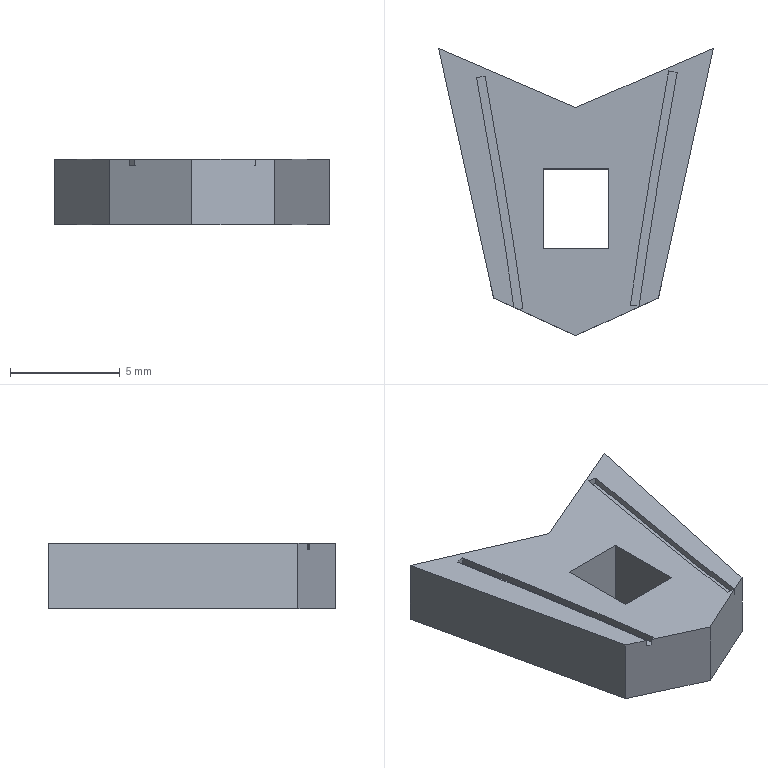Part | SolidWorks | features BaseBody 1 | 1 solid | 22 faces | box 12.536 x 13.11 x 3 mm | volume 276.053 mm3 | plane 18 | spline 4
STEP:
#1=CARTESIAN_POINT('',(2.822,-5.905,1.2));
#2=VERTEX_POINT('',#1);
#3=CARTESIAN_POINT('',(1.08,-16.586,1.2));
#4=VERTEX_POINT('',#3);
#5=CARTESIAN_POINT('',(2.822,-5.905,1.2));
#6=CARTESIAN_POINT('',(2.422,-8.09,1.2));
#7=CARTESIAN_POINT('',(1.593,-12.754,1.2));
#8=CARTESIAN_POINT('',(1.08,-16.586,1.2));
#9=B_SPLINE_CURVE_WITH_KNOTS('',3,(#5,#6,#7,#8),.UNSPECIFIED.,.F.,.F.,(4,4),(0.2382,0.9072),.UNSPECIFIED.);
#10=EDGE_CURVE('',#2,#4,#9,.T.);
#11=ORIENTED_EDGE('',*,*,#10,.T.);
#12=CARTESIAN_POINT('',(1.476,-16.639,1.2));
#13=VERTEX_POINT('',#12);
#14=CARTESIAN_POINT('',(1.476,-16.639,1.2));
#15=DIRECTION('',(-0.9911,0.1328,0.));
#16=VECTOR('',#15,1000.);
#17=LINE('',#14,#16);
#18=EDGE_CURVE('',#13,#4,#17,.T.);
#19=ORIENTED_EDGE('',*,*,#18,.F.);
#20=CARTESIAN_POINT('',(3.216,-5.977,1.2));
#21=VERTEX_POINT('',#20);
#22=CARTESIAN_POINT('',(3.216,-5.977,1.2));
#23=CARTESIAN_POINT('',(2.816,-8.159,1.2));
#24=CARTESIAN_POINT('',(1.988,-12.821,1.2));
#25=CARTESIAN_POINT('',(1.476,-16.639,1.2));
#26=B_SPLINE_CURVE_WITH_KNOTS('',3,(#22,#23,#24,#25),.UNSPECIFIED.,.F.,.F.,(4,4),(0.,1.),.UNSPECIFIED.);
#27=EDGE_CURVE('',#21,#13,#26,.T.);
#28=ORIENTED_EDGE('',*,*,#27,.F.);
#29=CARTESIAN_POINT('',(2.822,-5.905,1.2));
#30=DIRECTION('',(0.9837,-0.18,0.));
#31=VECTOR('',#30,1000.);
#32=LINE('',#29,#31);
#33=EDGE_CURVE('',#2,#21,#32,.T.);
#34=ORIENTED_EDGE('',*,*,#33,.F.);
#35=EDGE_LOOP('',(#11,#19,#28,#34));
#36=FACE_OUTER_BOUND('',#35,.T.);
#37=CARTESIAN_POINT('',(1.994,-10.628,1.2));
#38=DIRECTION('',(0.,0.,-1.));
#39=DIRECTION('',(0.,-1.,0.));
#40=AXIS2_PLACEMENT_3D('',#37,#38,#39);
#41=PLANE('',#40);
#42=ADVANCED_FACE('',(#36),#41,.F.);
#43=CARTESIAN_POINT('',(1.476,-16.639,1.5));
#44=VERTEX_POINT('',#43);
#45=CARTESIAN_POINT('',(1.08,-16.586,1.5));
#46=VERTEX_POINT('',#45);
#47=CARTESIAN_POINT('',(1.476,-16.639,1.5));
#48=DIRECTION('',(-0.9911,0.1328,0.));
#49=VECTOR('',#48,1000.);
#50=LINE('',#47,#49);
#51=EDGE_CURVE('',#44,#46,#50,.T.);
#52=ORIENTED_EDGE('',*,*,#51,.F.);
#53=CARTESIAN_POINT('',(1.476,-16.639,1.2));
#54=DIRECTION('',(0.,0.,1.));
#55=VECTOR('',#54,1000.);
#56=LINE('',#53,#55);
#57=EDGE_CURVE('',#13,#44,#56,.T.);
#58=ORIENTED_EDGE('',*,*,#57,.F.);
#59=ORIENTED_EDGE('',*,*,#18,.T.);
#60=CARTESIAN_POINT('',(1.08,-16.586,1.2));
#61=DIRECTION('',(0.,0.,1.));
#62=VECTOR('',#61,1000.);
#63=LINE('',#60,#62);
#64=EDGE_CURVE('',#4,#46,#63,.T.);
#65=ORIENTED_EDGE('',*,*,#64,.T.);
#66=EDGE_LOOP('',(#52,#58,#59,#65));
#67=FACE_OUTER_BOUND('',#66,.T.);
#68=CARTESIAN_POINT('',(1.476,-16.639,1.2));
#69=DIRECTION('',(0.1328,0.9911,0.));
#70=DIRECTION('',(0.,0.,-1.));
#71=AXIS2_PLACEMENT_3D('',#68,#69,#70);
#72=PLANE('',#71);
#73=ADVANCED_FACE('',(#67),#72,.T.);
#74=CARTESIAN_POINT('',(3.216,-5.977,1.5));
#75=VERTEX_POINT('',#74);
#76=CARTESIAN_POINT('',(3.216,-5.977,1.5));
#77=CARTESIAN_POINT('',(2.816,-8.159,1.5));
#78=CARTESIAN_POINT('',(1.988,-12.821,1.5));
#79=CARTESIAN_POINT('',(1.476,-16.639,1.5));
#80=B_SPLINE_CURVE_WITH_KNOTS('',3,(#76,#77,#78,#79),.UNSPECIFIED.,.F.,.F.,(4,4),(0.,1.),.UNSPECIFIED.);
#81=EDGE_CURVE('',#75,#44,#80,.T.);
#82=ORIENTED_EDGE('',*,*,#81,.F.);
#83=CARTESIAN_POINT('',(3.216,-5.977,1.2));
#84=DIRECTION('',(0.,0.,1.));
#85=VECTOR('',#84,1000.);
#86=LINE('',#83,#85);
#87=EDGE_CURVE('',#21,#75,#86,.T.);
#88=ORIENTED_EDGE('',*,*,#87,.F.);
#89=ORIENTED_EDGE('',*,*,#27,.T.);
#90=ORIENTED_EDGE('',*,*,#57,.T.);
#91=EDGE_LOOP('',(#82,#88,#89,#90));
#92=FACE_OUTER_BOUND('',#91,.T.);
#93=CARTESIAN_POINT('',(3.216,-5.977,1.2));
#94=CARTESIAN_POINT('',(3.216,-5.977,1.5));
#95=CARTESIAN_POINT('',(2.816,-8.159,1.2));
#96=CARTESIAN_POINT('',(2.816,-8.159,1.5));
#97=CARTESIAN_POINT('',(1.988,-12.821,1.2));
#98=CARTESIAN_POINT('',(1.988,-12.821,1.5));
#99=CARTESIAN_POINT('',(1.476,-16.639,1.2));
#100=CARTESIAN_POINT('',(1.476,-16.639,1.5));
#101=B_SPLINE_SURFACE_WITH_KNOTS('',3,1,((#93,#94),(#95,#96),(#97,#98),(#99,#100)),.UNSPECIFIED.,.F.,.F.,.F.,(4,4),(2,2),(0.,1.),(0.,1.),.UNSPECIFIED.);
#102=ADVANCED_FACE('',(#92),#101,.T.);
#103=CARTESIAN_POINT('',(2.822,-5.905,1.5));
#104=VERTEX_POINT('',#103);
#105=CARTESIAN_POINT('',(2.822,-5.905,1.5));
#106=DIRECTION('',(0.9837,-0.18,0.));
#107=VECTOR('',#106,1000.);
#108=LINE('',#105,#107);
#109=EDGE_CURVE('',#104,#75,#108,.T.);
#110=ORIENTED_EDGE('',*,*,#109,.F.);
#111=CARTESIAN_POINT('',(2.822,-5.905,1.2));
#112=DIRECTION('',(0.,0.,1.));
#113=VECTOR('',#112,1000.);
#114=LINE('',#111,#113);
#115=EDGE_CURVE('',#2,#104,#114,.T.);
#116=ORIENTED_EDGE('',*,*,#115,.F.);
#117=ORIENTED_EDGE('',*,*,#33,.T.);
#118=ORIENTED_EDGE('',*,*,#87,.T.);
#119=EDGE_LOOP('',(#110,#116,#117,#118));
#120=FACE_OUTER_BOUND('',#119,.T.);
#121=CARTESIAN_POINT('',(2.822,-5.905,1.2));
#122=DIRECTION('',(-0.18,-0.9837,0.));
#123=DIRECTION('',(-0.9837,0.18,0.));
#124=AXIS2_PLACEMENT_3D('',#121,#122,#123);
#125=PLANE('',#124);
#126=ADVANCED_FACE('',(#120),#125,.T.);
#127=CARTESIAN_POINT('',(2.822,-5.905,1.5));
#128=CARTESIAN_POINT('',(2.422,-8.09,1.5));
#129=CARTESIAN_POINT('',(1.593,-12.754,1.5));
#130=CARTESIAN_POINT('',(1.08,-16.586,1.5));
#131=B_SPLINE_CURVE_WITH_KNOTS('',3,(#127,#128,#129,#130),.UNSPECIFIED.,.F.,.F.,(4,4),(0.2382,0.9072),.UNSPECIFIED.);
#132=EDGE_CURVE('',#104,#46,#131,.T.);
#133=ORIENTED_EDGE('',*,*,#132,.T.);
#134=ORIENTED_EDGE('',*,*,#64,.F.);
#135=ORIENTED_EDGE('',*,*,#10,.F.);
#136=ORIENTED_EDGE('',*,*,#115,.T.);
#137=EDGE_LOOP('',(#133,#134,#135,#136));
#138=FACE_OUTER_BOUND('',#137,.T.);
#139=CARTESIAN_POINT('',(2.822,-5.905,1.2));
#140=CARTESIAN_POINT('',(2.822,-5.905,1.5));
#141=CARTESIAN_POINT('',(2.422,-8.09,1.2));
#142=CARTESIAN_POINT('',(2.422,-8.09,1.5));
#143=CARTESIAN_POINT('',(1.593,-12.754,1.2));
#144=CARTESIAN_POINT('',(1.593,-12.754,1.5));
#145=CARTESIAN_POINT('',(1.08,-16.586,1.2));
#146=CARTESIAN_POINT('',(1.08,-16.586,1.5));
#147=B_SPLINE_SURFACE_WITH_KNOTS('',3,1,((#139,#140),(#141,#142),(#143,#144),(#145,#146)),.UNSPECIFIED.,.F.,.F.,.F.,(4,4),(2,2),(0.2382,0.9072),(0.,1.),.UNSPECIFIED.);
#148=ADVANCED_FACE('',(#138),#147,.F.);
#149=CARTESIAN_POINT('',(-5.546,-6.138,1.5));
#150=VERTEX_POINT('',#149);
#151=CARTESIAN_POINT('',(-3.824,-16.751,1.5));
#152=VERTEX_POINT('',#151);
#153=CARTESIAN_POINT('',(-5.546,-6.138,1.5));
#154=CARTESIAN_POINT('',(-5.126,-8.442,1.5));
#155=CARTESIAN_POINT('',(-4.318,-13.02,1.5));
#156=CARTESIAN_POINT('',(-3.824,-16.751,1.5));
#157=B_SPLINE_CURVE_WITH_KNOTS('',3,(#153,#154,#155,#156),.UNSPECIFIED.,.F.,.F.,(4,4),(0.2611,0.9169),.UNSPECIFIED.);
#158=EDGE_CURVE('',#150,#152,#157,.T.);
#159=ORIENTED_EDGE('',*,*,#158,.F.);
#160=CARTESIAN_POINT('',(-5.546,-6.138,1.2));
#161=VERTEX_POINT('',#160);
#162=CARTESIAN_POINT('',(-5.546,-6.138,1.2));
#163=DIRECTION('',(0.,0.,1.));
#164=VECTOR('',#163,1000.);
#165=LINE('',#162,#164);
#166=EDGE_CURVE('',#161,#150,#165,.T.);
#167=ORIENTED_EDGE('',*,*,#166,.F.);
#168=CARTESIAN_POINT('',(-3.824,-16.751,1.2));
#169=VERTEX_POINT('',#168);
#170=CARTESIAN_POINT('',(-5.546,-6.138,1.2));
#171=CARTESIAN_POINT('',(-5.126,-8.442,1.2));
#172=CARTESIAN_POINT('',(-4.318,-13.02,1.2));
#173=CARTESIAN_POINT('',(-3.824,-16.751,1.2));
#174=B_SPLINE_CURVE_WITH_KNOTS('',3,(#170,#171,#172,#173),.UNSPECIFIED.,.F.,.F.,(4,4),(0.2611,0.9169),.UNSPECIFIED.);
#175=EDGE_CURVE('',#161,#169,#174,.T.);
#176=ORIENTED_EDGE('',*,*,#175,.T.);
#177=CARTESIAN_POINT('',(-3.824,-16.751,1.2));
#178=DIRECTION('',(0.,0.,1.));
#179=VECTOR('',#178,1000.);
#180=LINE('',#177,#179);
#181=EDGE_CURVE('',#169,#152,#180,.T.);
#182=ORIENTED_EDGE('',*,*,#181,.T.);
#183=EDGE_LOOP('',(#159,#167,#176,#182));
#184=FACE_OUTER_BOUND('',#183,.T.);
#185=CARTESIAN_POINT('',(-5.546,-6.138,1.2));
#186=CARTESIAN_POINT('',(-5.546,-6.138,1.5));
#187=CARTESIAN_POINT('',(-5.126,-8.442,1.2));
#188=CARTESIAN_POINT('',(-5.126,-8.442,1.5));
#189=CARTESIAN_POINT('',(-4.318,-13.02,1.2));
#190=CARTESIAN_POINT('',(-4.318,-13.02,1.5));
#191=CARTESIAN_POINT('',(-3.824,-16.751,1.2));
#192=CARTESIAN_POINT('',(-3.824,-16.751,1.5));
#193=B_SPLINE_SURFACE_WITH_KNOTS('',3,1,((#185,#186),(#187,#188),(#189,#190),(#191,#192)),.UNSPECIFIED.,.F.,.F.,.F.,(4,4),(2,2),(0.2611,0.9169),(0.,1.),.UNSPECIFIED.);
#194=ADVANCED_FACE('',(#184),#193,.T.);
#195=CARTESIAN_POINT('',(-5.939,-6.21,1.5));
#196=VERTEX_POINT('',#195);
#197=CARTESIAN_POINT('',(-5.939,-6.21,1.5));
#198=DIRECTION('',(0.9838,0.1793,0.));
#199=VECTOR('',#198,1000.);
#200=LINE('',#197,#199);
#201=EDGE_CURVE('',#196,#150,#200,.T.);
#202=ORIENTED_EDGE('',*,*,#201,.F.);
#203=CARTESIAN_POINT('',(-5.939,-6.21,1.2));
#204=VERTEX_POINT('',#203);
#205=CARTESIAN_POINT('',(-5.939,-6.21,1.2));
#206=DIRECTION('',(0.,0.,1.));
#207=VECTOR('',#206,1000.);
#208=LINE('',#205,#207);
#209=EDGE_CURVE('',#204,#196,#208,.T.);
#210=ORIENTED_EDGE('',*,*,#209,.F.);
#211=CARTESIAN_POINT('',(-5.939,-6.21,1.2));
#212=DIRECTION('',(0.9838,0.1793,0.));
#213=VECTOR('',#212,1000.);
#214=LINE('',#211,#213);
#215=EDGE_CURVE('',#204,#161,#214,.T.);
#216=ORIENTED_EDGE('',*,*,#215,.T.);
#217=ORIENTED_EDGE('',*,*,#166,.T.);
#218=EDGE_LOOP('',(#202,#210,#216,#217));
#219=FACE_OUTER_BOUND('',#218,.T.);
#220=CARTESIAN_POINT('',(-5.939,-6.21,1.2));
#221=DIRECTION('',(0.1793,-0.9838,0.));
#222=DIRECTION('',(0.,0.,-1.));
#223=AXIS2_PLACEMENT_3D('',#220,#221,#222);
#224=PLANE('',#223);
#225=ADVANCED_FACE('',(#219),#224,.T.);
#226=CARTESIAN_POINT('',(-4.237,-16.683,1.2));
#227=VERTEX_POINT('',#226);
#228=CARTESIAN_POINT('',(-4.029,-16.778,1.2));
#229=VERTEX_POINT('',#228);
#230=CARTESIAN_POINT('',(-1.413,-17.978,1.2));
#231=DIRECTION('',(0.9089,-0.4171,0.));
#232=VECTOR('',#231,1000.);
#233=LINE('',#230,#232);
#234=EDGE_CURVE('',#227,#229,#233,.T.);
#235=ORIENTED_EDGE('',*,*,#234,.T.);
#236=CARTESIAN_POINT('',(-3.824,-16.751,1.2));
#237=DIRECTION('',(-0.9913,-0.1313,0.));
#238=VECTOR('',#237,1000.);
#239=LINE('',#236,#238);
#240=EDGE_CURVE('',#169,#229,#239,.T.);
#241=ORIENTED_EDGE('',*,*,#240,.F.);
#242=ORIENTED_EDGE('',*,*,#175,.F.);
#243=ORIENTED_EDGE('',*,*,#215,.F.);
#244=CARTESIAN_POINT('',(-5.939,-6.21,1.2));
#245=CARTESIAN_POINT('',(-5.524,-8.486,1.2));
#246=CARTESIAN_POINT('',(-4.73,-12.988,1.2));
#247=CARTESIAN_POINT('',(-4.237,-16.683,1.2));
#248=B_SPLINE_CURVE_WITH_KNOTS('',3,(#244,#245,#246,#247),.UNSPECIFIED.,.F.,.F.,(4,4),(0.,0.9892),.UNSPECIFIED.);
#249=EDGE_CURVE('',#204,#227,#248,.T.);
#250=ORIENTED_EDGE('',*,*,#249,.T.);
#251=EDGE_LOOP('',(#235,#241,#242,#243,#250));
#252=FACE_OUTER_BOUND('',#251,.T.);
#253=CARTESIAN_POINT('',(-5.107,-10.976,1.2));
#254=DIRECTION('',(0.,0.,1.));
#255=DIRECTION('',(1.,0.,0.));
#256=AXIS2_PLACEMENT_3D('',#253,#254,#255);
#257=PLANE('',#256);
#258=ADVANCED_FACE('',(#252),#257,.T.);
#259=CARTESIAN_POINT('',(-4.029,-16.778,1.5));
#260=VERTEX_POINT('',#259);
#261=CARTESIAN_POINT('',(-4.029,-16.778,1.5));
#262=DIRECTION('',(0.,0.,1.));
#263=VECTOR('',#262,1000.);
#264=LINE('',#261,#263);
#265=EDGE_CURVE('',#229,#260,#264,.T.);
#266=ORIENTED_EDGE('',*,*,#265,.T.);
#267=CARTESIAN_POINT('',(-3.824,-16.751,1.5));
#268=DIRECTION('',(-0.9913,-0.1313,0.));
#269=VECTOR('',#268,1000.);
#270=LINE('',#267,#269);
#271=EDGE_CURVE('',#152,#260,#270,.T.);
#272=ORIENTED_EDGE('',*,*,#271,.F.);
#273=ORIENTED_EDGE('',*,*,#181,.F.);
#274=ORIENTED_EDGE('',*,*,#240,.T.);
#275=EDGE_LOOP('',(#266,#272,#273,#274));
#276=FACE_OUTER_BOUND('',#275,.T.);
#277=CARTESIAN_POINT('',(-3.824,-16.751,1.2));
#278=DIRECTION('',(-0.1313,0.9913,0.));
#279=DIRECTION('',(0.,0.,1.));
#280=AXIS2_PLACEMENT_3D('',#277,#278,#279);
#281=PLANE('',#280);
#282=ADVANCED_FACE('',(#276),#281,.T.);
#283=ORIENTED_EDGE('',*,*,#249,.F.);
#284=ORIENTED_EDGE('',*,*,#209,.T.);
#285=CARTESIAN_POINT('',(-4.237,-16.683,1.5));
#286=VERTEX_POINT('',#285);
#287=CARTESIAN_POINT('',(-5.939,-6.21,1.5));
#288=CARTESIAN_POINT('',(-5.524,-8.486,1.5));
#289=CARTESIAN_POINT('',(-4.73,-12.988,1.5));
#290=CARTESIAN_POINT('',(-4.237,-16.683,1.5));
#291=B_SPLINE_CURVE_WITH_KNOTS('',3,(#287,#288,#289,#290),.UNSPECIFIED.,.F.,.F.,(4,4),(0.,0.9892),.UNSPECIFIED.);
#292=EDGE_CURVE('',#196,#286,#291,.T.);
#293=ORIENTED_EDGE('',*,*,#292,.T.);
#294=CARTESIAN_POINT('',(-4.237,-16.683,1.2));
#295=DIRECTION('',(0.,0.,1.));
#296=VECTOR('',#295,1000.);
#297=LINE('',#294,#296);
#298=EDGE_CURVE('',#227,#286,#297,.T.);
#299=ORIENTED_EDGE('',*,*,#298,.F.);
#300=EDGE_LOOP('',(#283,#284,#293,#299));
#301=FACE_OUTER_BOUND('',#300,.T.);
#302=CARTESIAN_POINT('',(-5.939,-6.21,1.2));
#303=CARTESIAN_POINT('',(-5.939,-6.21,1.5));
#304=CARTESIAN_POINT('',(-5.524,-8.486,1.2));
#305=CARTESIAN_POINT('',(-5.524,-8.486,1.5));
#306=CARTESIAN_POINT('',(-4.73,-12.988,1.2));
#307=CARTESIAN_POINT('',(-4.73,-12.988,1.5));
#308=CARTESIAN_POINT('',(-4.237,-16.683,1.2));
#309=CARTESIAN_POINT('',(-4.237,-16.683,1.5));
#310=B_SPLINE_SURFACE_WITH_KNOTS('',3,1,((#302,#303),(#304,#305),(#306,#307),(#308,#309)),.UNSPECIFIED.,.F.,.F.,.F.,(4,4),(2,2),(0.,0.9892),(0.,1.),.UNSPECIFIED.);
#311=ADVANCED_FACE('',(#301),#310,.F.);
#312=CARTESIAN_POINT('',(0.0944,-10.374,-1.5));
#313=VERTEX_POINT('',#312);
#314=CARTESIAN_POINT('',(-2.901,-10.374,-1.5));
#315=VERTEX_POINT('',#314);
#316=CARTESIAN_POINT('',(0.0944,-10.374,-1.5));
#317=DIRECTION('',(-1.,0.,0.));
#318=VECTOR('',#317,1000.);
#319=LINE('',#316,#318);
#320=EDGE_CURVE('',#313,#315,#319,.T.);
#321=ORIENTED_EDGE('',*,*,#320,.F.);
#322=CARTESIAN_POINT('',(0.0944,-10.374,1.5));
#323=VERTEX_POINT('',#322);
#324=CARTESIAN_POINT('',(0.0944,-10.374,1.5));
#325=DIRECTION('',(0.,0.,-1.));
#326=VECTOR('',#325,1000.);
#327=LINE('',#324,#326);
#328=EDGE_CURVE('',#323,#313,#327,.T.);
#329=ORIENTED_EDGE('',*,*,#328,.F.);
#330=CARTESIAN_POINT('',(-2.901,-10.374,1.5));
#331=VERTEX_POINT('',#330);
#332=CARTESIAN_POINT('',(0.0944,-10.374,1.5));
#333=DIRECTION('',(-1.,0.,0.));
#334=VECTOR('',#333,1000.);
#335=LINE('',#332,#334);
#336=EDGE_CURVE('',#323,#331,#335,.T.);
#337=ORIENTED_EDGE('',*,*,#336,.T.);
#338=CARTESIAN_POINT('',(-2.901,-10.374,1.5));
#339=DIRECTION('',(0.,0.,-1.));
#340=VECTOR('',#339,1000.);
#341=LINE('',#338,#340);
#342=EDGE_CURVE('',#331,#315,#341,.T.);
#343=ORIENTED_EDGE('',*,*,#342,.T.);
#344=EDGE_LOOP('',(#321,#329,#337,#343));
#345=FACE_OUTER_BOUND('',#344,.T.);
#346=CARTESIAN_POINT('',(0.0944,-10.374,1.5));
#347=DIRECTION('',(0.,-1.,0.));
#348=DIRECTION('',(0.,0.,-1.));
#349=AXIS2_PLACEMENT_3D('',#346,#347,#348);
#350=PLANE('',#349);
#351=ADVANCED_FACE('',(#345),#350,.T.);
#352=CARTESIAN_POINT('',(0.0944,-13.997,-1.5));
#353=VERTEX_POINT('',#352);
#354=CARTESIAN_POINT('',(0.0944,-13.997,-1.5));
#355=DIRECTION('',(0.,1.,0.));
#356=VECTOR('',#355,1000.);
#357=LINE('',#354,#356);
#358=EDGE_CURVE('',#353,#313,#357,.T.);
#359=ORIENTED_EDGE('',*,*,#358,.F.);
#360=CARTESIAN_POINT('',(0.0944,-13.997,1.5));
#361=VERTEX_POINT('',#360);
#362=CARTESIAN_POINT('',(0.0944,-13.997,1.5));
#363=DIRECTION('',(0.,0.,-1.));
#364=VECTOR('',#363,1000.);
#365=LINE('',#362,#364);
#366=EDGE_CURVE('',#361,#353,#365,.T.);
#367=ORIENTED_EDGE('',*,*,#366,.F.);
#368=CARTESIAN_POINT('',(0.0944,-13.997,1.5));
#369=DIRECTION('',(0.,1.,0.));
#370=VECTOR('',#369,1000.);
#371=LINE('',#368,#370);
#372=EDGE_CURVE('',#361,#323,#371,.T.);
#373=ORIENTED_EDGE('',*,*,#372,.T.);
#374=ORIENTED_EDGE('',*,*,#328,.T.);
#375=EDGE_LOOP('',(#359,#367,#373,#374));
#376=FACE_OUTER_BOUND('',#375,.T.);
#377=CARTESIAN_POINT('',(0.0944,-13.997,1.5));
#378=DIRECTION('',(-1.,0.,0.));
#379=DIRECTION('',(0.,0.,1.));
#380=AXIS2_PLACEMENT_3D('',#377,#378,#379);
#381=PLANE('',#380);
#382=ADVANCED_FACE('',(#376),#381,.T.);
#383=CARTESIAN_POINT('',(-2.901,-13.997,-1.5));
#384=VERTEX_POINT('',#383);
#385=CARTESIAN_POINT('',(-2.901,-13.997,-1.5));
#386=DIRECTION('',(1.,0.,0.));
#387=VECTOR('',#386,1000.);
#388=LINE('',#385,#387);
#389=EDGE_CURVE('',#384,#353,#388,.T.);
#390=ORIENTED_EDGE('',*,*,#389,.F.);
#391=CARTESIAN_POINT('',(-2.901,-13.997,1.5));
#392=VERTEX_POINT('',#391);
#393=CARTESIAN_POINT('',(-2.901,-13.997,1.5));
#394=DIRECTION('',(0.,0.,-1.));
#395=VECTOR('',#394,1000.);
#396=LINE('',#393,#395);
#397=EDGE_CURVE('',#392,#384,#396,.T.);
#398=ORIENTED_EDGE('',*,*,#397,.F.);
#399=CARTESIAN_POINT('',(-2.901,-13.997,1.5));
#400=DIRECTION('',(1.,0.,0.));
#401=VECTOR('',#400,1000.);
#402=LINE('',#399,#401);
#403=EDGE_CURVE('',#392,#361,#402,.T.);
#404=ORIENTED_EDGE('',*,*,#403,.T.);
#405=ORIENTED_EDGE('',*,*,#366,.T.);
#406=EDGE_LOOP('',(#390,#398,#404,#405));
#407=FACE_OUTER_BOUND('',#406,.T.);
#408=CARTESIAN_POINT('',(-2.901,-13.997,1.5));
#409=DIRECTION('',(0.,1.,0.));
#410=DIRECTION('',(1.,0.,0.));
#411=AXIS2_PLACEMENT_3D('',#408,#409,#410);
#412=PLANE('',#411);
#413=ADVANCED_FACE('',(#407),#412,.T.);
#414=CARTESIAN_POINT('',(-2.901,-10.374,-1.5));
#415=DIRECTION('',(0.,-1.,0.));
#416=VECTOR('',#415,1000.);
#417=LINE('',#414,#416);
#418=EDGE_CURVE('',#315,#384,#417,.T.);
#419=ORIENTED_EDGE('',*,*,#418,.F.);
#420=ORIENTED_EDGE('',*,*,#342,.F.);
#421=CARTESIAN_POINT('',(-2.901,-10.374,1.5));
#422=DIRECTION('',(0.,-1.,0.));
#423=VECTOR('',#422,1000.);
#424=LINE('',#421,#423);
#425=EDGE_CURVE('',#331,#392,#424,.T.);
#426=ORIENTED_EDGE('',*,*,#425,.T.);
#427=ORIENTED_EDGE('',*,*,#397,.T.);
#428=EDGE_LOOP('',(#419,#420,#426,#427));
#429=FACE_OUTER_BOUND('',#428,.T.);
#430=CARTESIAN_POINT('',(-2.901,-10.374,1.5));
#431=DIRECTION('',(1.,0.,0.));
#432=DIRECTION('',(0.,1.,0.));
#433=AXIS2_PLACEMENT_3D('',#430,#431,#432);
#434=PLANE('',#433);
#435=ADVANCED_FACE('',(#429),#434,.T.);
#436=CARTESIAN_POINT('',(-1.413,-17.978,-1.5));
#437=VERTEX_POINT('',#436);
#438=CARTESIAN_POINT('',(2.358,-16.258,-1.5));
#439=VERTEX_POINT('',#438);
#440=CARTESIAN_POINT('',(2.358,-16.258,-1.5));
#441=DIRECTION('',(0.9098,0.415,0.));
#442=VECTOR('',#441,1000.);
#443=LINE('',#440,#442);
#444=EDGE_CURVE('',#437,#439,#443,.T.);
#445=ORIENTED_EDGE('',*,*,#444,.T.);
#446=CARTESIAN_POINT('',(2.358,-16.258,1.5));
#447=VERTEX_POINT('',#446);
#448=CARTESIAN_POINT('',(2.358,-16.258,1.5));
#449=DIRECTION('',(0.,0.,-1.));
#450=VECTOR('',#449,1000.);
#451=LINE('',#448,#450);
#452=EDGE_CURVE('',#447,#439,#451,.T.);
#453=ORIENTED_EDGE('',*,*,#452,.F.);
#454=CARTESIAN_POINT('',(-1.413,-17.978,1.5));
#455=VERTEX_POINT('',#454);
#456=CARTESIAN_POINT('',(2.358,-16.258,1.5));
#457=DIRECTION('',(0.9098,0.415,0.));
#458=VECTOR('',#457,1000.);
#459=LINE('',#456,#458);
#460=EDGE_CURVE('',#455,#447,#459,.T.);
#461=ORIENTED_EDGE('',*,*,#460,.F.);
#462=CARTESIAN_POINT('',(-1.413,-17.978,1.5));
#463=DIRECTION('',(0.,0.,-1.));
#464=VECTOR('',#463,1000.);
#465=LINE('',#462,#464);
#466=EDGE_CURVE('',#455,#437,#465,.T.);
#467=ORIENTED_EDGE('',*,*,#466,.T.);
#468=EDGE_LOOP('',(#445,#453,#461,#467));
#469=FACE_OUTER_BOUND('',#468,.T.);
#470=CARTESIAN_POINT('',(2.358,-16.258,1.5));
#471=DIRECTION('',(-0.415,0.9098,0.));
#472=DIRECTION('',(0.,0.,1.));
#473=AXIS2_PLACEMENT_3D('',#470,#471,#472);
#474=PLANE('',#473);
#475=ADVANCED_FACE('',(#469),#474,.F.);
#476=ORIENTED_EDGE('',*,*,#234,.F.);
#477=ORIENTED_EDGE('',*,*,#298,.T.);
#478=CARTESIAN_POINT('',(-5.162,-16.258,1.5));
#479=VERTEX_POINT('',#478);
#480=CARTESIAN_POINT('',(-1.413,-17.978,1.5));
#481=DIRECTION('',(0.9089,-0.4171,0.));
#482=VECTOR('',#481,1000.);
#483=LINE('',#480,#482);
#484=EDGE_CURVE('',#479,#286,#483,.T.);
#485=ORIENTED_EDGE('',*,*,#484,.F.);
#486=CARTESIAN_POINT('',(-5.162,-16.258,-1.5));
#487=VERTEX_POINT('',#486);
#488=CARTESIAN_POINT('',(-5.162,-16.258,1.5));
#489=DIRECTION('',(0.,0.,-1.));
#490=VECTOR('',#489,1000.);
#491=LINE('',#488,#490);
#492=EDGE_CURVE('',#479,#487,#491,.T.);
#493=ORIENTED_EDGE('',*,*,#492,.T.);
#494=CARTESIAN_POINT('',(-1.413,-17.978,-1.5));
#495=DIRECTION('',(0.9089,-0.4171,0.));
#496=VECTOR('',#495,1000.);
#497=LINE('',#494,#496);
#498=EDGE_CURVE('',#487,#437,#497,.T.);
#499=ORIENTED_EDGE('',*,*,#498,.T.);
#500=ORIENTED_EDGE('',*,*,#466,.F.);
#501=CARTESIAN_POINT('',(-1.413,-17.978,1.5));
#502=DIRECTION('',(0.9089,-0.4171,0.));
#503=VECTOR('',#502,1000.);
#504=LINE('',#501,#503);
#505=EDGE_CURVE('',#260,#455,#504,.T.);
#506=ORIENTED_EDGE('',*,*,#505,.F.);
#507=ORIENTED_EDGE('',*,*,#265,.F.);
#508=EDGE_LOOP('',(#476,#477,#485,#493,#499,#500,#506,#507));
#509=FACE_OUTER_BOUND('',#508,.T.);
#510=CARTESIAN_POINT('',(-1.413,-17.978,1.5));
#511=DIRECTION('',(0.4171,0.9089,0.));
#512=DIRECTION('',(0.,0.,-1.));
#513=AXIS2_PLACEMENT_3D('',#510,#511,#512);
#514=PLANE('',#513);
#515=ADVANCED_FACE('',(#509),#514,.F.);
#516=CARTESIAN_POINT('',(-7.67,-4.868,-1.5));
#517=VERTEX_POINT('',#516);
#518=CARTESIAN_POINT('',(-5.162,-16.258,-1.5));
#519=DIRECTION('',(0.215,-0.9766,0.));
#520=VECTOR('',#519,1000.);
#521=LINE('',#518,#520);
#522=EDGE_CURVE('',#517,#487,#521,.T.);
#523=ORIENTED_EDGE('',*,*,#522,.T.);
#524=ORIENTED_EDGE('',*,*,#492,.F.);
#525=CARTESIAN_POINT('',(-7.67,-4.868,1.5));
#526=VERTEX_POINT('',#525);
#527=CARTESIAN_POINT('',(-5.162,-16.258,1.5));
#528=DIRECTION('',(0.215,-0.9766,0.));
#529=VECTOR('',#528,1000.);
#530=LINE('',#527,#529);
#531=EDGE_CURVE('',#526,#479,#530,.T.);
#532=ORIENTED_EDGE('',*,*,#531,.F.);
#533=CARTESIAN_POINT('',(-7.67,-4.868,1.5));
#534=DIRECTION('',(0.,0.,-1.));
#535=VECTOR('',#534,1000.);
#536=LINE('',#533,#535);
#537=EDGE_CURVE('',#526,#517,#536,.T.);
#538=ORIENTED_EDGE('',*,*,#537,.T.);
#539=EDGE_LOOP('',(#523,#524,#532,#538));
#540=FACE_OUTER_BOUND('',#539,.T.);
#541=CARTESIAN_POINT('',(-5.162,-16.258,1.5));
#542=DIRECTION('',(0.9766,0.215,0.));
#543=DIRECTION('',(0.,0.,-1.));
#544=AXIS2_PLACEMENT_3D('',#541,#542,#543);
#545=PLANE('',#544);
#546=ADVANCED_FACE('',(#540),#545,.F.);
#547=CARTESIAN_POINT('',(-1.413,-7.574,-1.5));
#548=VERTEX_POINT('',#547);
#549=CARTESIAN_POINT('',(-7.67,-4.868,-1.5));
#550=DIRECTION('',(-0.9179,0.3969,0.));
#551=VECTOR('',#550,1000.);
#552=LINE('',#549,#551);
#553=EDGE_CURVE('',#548,#517,#552,.T.);
#554=ORIENTED_EDGE('',*,*,#553,.T.);
#555=ORIENTED_EDGE('',*,*,#537,.F.);
#556=CARTESIAN_POINT('',(-1.413,-7.574,1.5));
#557=VERTEX_POINT('',#556);
#558=CARTESIAN_POINT('',(-7.67,-4.868,1.5));
#559=DIRECTION('',(-0.9179,0.3969,0.));
#560=VECTOR('',#559,1000.);
#561=LINE('',#558,#560);
#562=EDGE_CURVE('',#557,#526,#561,.T.);
#563=ORIENTED_EDGE('',*,*,#562,.F.);
#564=CARTESIAN_POINT('',(-1.413,-7.574,1.5));
#565=DIRECTION('',(0.,0.,-1.));
#566=VECTOR('',#565,1000.);
#567=LINE('',#564,#566);
#568=EDGE_CURVE('',#557,#548,#567,.T.);
#569=ORIENTED_EDGE('',*,*,#568,.T.);
#570=EDGE_LOOP('',(#554,#555,#563,#569));
#571=FACE_OUTER_BOUND('',#570,.T.);
#572=CARTESIAN_POINT('',(-7.67,-4.868,1.5));
#573=DIRECTION('',(-0.3969,-0.9179,0.));
#574=DIRECTION('',(-0.9179,0.3969,0.));
#575=AXIS2_PLACEMENT_3D('',#572,#573,#574);
#576=PLANE('',#575);
#577=ADVANCED_FACE('',(#571),#576,.F.);
#578=CARTESIAN_POINT('',(4.866,-4.869,-1.5));
#579=VERTEX_POINT('',#578);
#580=CARTESIAN_POINT('',(-1.413,-7.574,-1.5));
#581=DIRECTION('',(-0.9184,-0.3957,0.));
#582=VECTOR('',#581,1000.);
#583=LINE('',#580,#582);
#584=EDGE_CURVE('',#579,#548,#583,.T.);
#585=ORIENTED_EDGE('',*,*,#584,.T.);
#586=ORIENTED_EDGE('',*,*,#568,.F.);
#587=CARTESIAN_POINT('',(4.866,-4.869,1.5));
#588=VERTEX_POINT('',#587);
#589=CARTESIAN_POINT('',(-1.413,-7.574,1.5));
#590=DIRECTION('',(-0.9184,-0.3957,0.));
#591=VECTOR('',#590,1000.);
#592=LINE('',#589,#591);
#593=EDGE_CURVE('',#588,#557,#592,.T.);
#594=ORIENTED_EDGE('',*,*,#593,.F.);
#595=CARTESIAN_POINT('',(4.866,-4.869,1.5));
#596=DIRECTION('',(0.,0.,-1.));
#597=VECTOR('',#596,1000.);
#598=LINE('',#595,#597);
#599=EDGE_CURVE('',#588,#579,#598,.T.);
#600=ORIENTED_EDGE('',*,*,#599,.T.);
#601=EDGE_LOOP('',(#585,#586,#594,#600));
#602=FACE_OUTER_BOUND('',#601,.T.);
#603=CARTESIAN_POINT('',(-1.413,-7.574,1.5));
#604=DIRECTION('',(0.3957,-0.9184,0.));
#605=DIRECTION('',(0.,0.,-1.));
#606=AXIS2_PLACEMENT_3D('',#603,#604,#605);
#607=PLANE('',#606);
#608=ADVANCED_FACE('',(#602),#607,.F.);
#609=CARTESIAN_POINT('',(4.866,-4.869,-1.5));
#610=DIRECTION('',(0.215,0.9766,0.));
#611=VECTOR('',#610,1000.);
#612=LINE('',#609,#611);
#613=EDGE_CURVE('',#439,#579,#612,.T.);
#614=ORIENTED_EDGE('',*,*,#613,.T.);
#615=ORIENTED_EDGE('',*,*,#599,.F.);
#616=CARTESIAN_POINT('',(4.866,-4.869,1.5));
#617=DIRECTION('',(0.215,0.9766,0.));
#618=VECTOR('',#617,1000.);
#619=LINE('',#616,#618);
#620=EDGE_CURVE('',#447,#588,#619,.T.);
#621=ORIENTED_EDGE('',*,*,#620,.F.);
#622=ORIENTED_EDGE('',*,*,#452,.T.);
#623=EDGE_LOOP('',(#614,#615,#621,#622));
#624=FACE_OUTER_BOUND('',#623,.T.);
#625=CARTESIAN_POINT('',(4.866,-4.869,1.5));
#626=DIRECTION('',(-0.9766,0.215,0.));
#627=DIRECTION('',(0.,0.,1.));
#628=AXIS2_PLACEMENT_3D('',#625,#626,#627);
#629=PLANE('',#628);
#630=ADVANCED_FACE('',(#624),#629,.F.);
#631=ORIENTED_EDGE('',*,*,#418,.T.);
#632=ORIENTED_EDGE('',*,*,#389,.T.);
#633=ORIENTED_EDGE('',*,*,#358,.T.);
#634=ORIENTED_EDGE('',*,*,#320,.T.);
#635=EDGE_LOOP('',(#631,#632,#633,#634));
#636=FACE_BOUND('',#635,.T.);
#637=ORIENTED_EDGE('',*,*,#613,.F.);
#638=ORIENTED_EDGE('',*,*,#444,.F.);
#639=ORIENTED_EDGE('',*,*,#498,.F.);
#640=ORIENTED_EDGE('',*,*,#522,.F.);
#641=ORIENTED_EDGE('',*,*,#553,.F.);
#642=ORIENTED_EDGE('',*,*,#584,.F.);
#643=EDGE_LOOP('',(#637,#638,#639,#640,#641,#642));
#644=FACE_OUTER_BOUND('',#643,.T.);
#645=CARTESIAN_POINT('',(0.,0.,-1.5));
#646=DIRECTION('',(0.,0.,1.));
#647=DIRECTION('',(1.,0.,0.));
#648=AXIS2_PLACEMENT_3D('',#645,#646,#647);
#649=PLANE('',#648);
#650=ADVANCED_FACE('',(#636,#644),#649,.F.);
#651=ORIENTED_EDGE('',*,*,#403,.F.);
#652=ORIENTED_EDGE('',*,*,#425,.F.);
#653=ORIENTED_EDGE('',*,*,#336,.F.);
#654=ORIENTED_EDGE('',*,*,#372,.F.);
#655=EDGE_LOOP('',(#651,#652,#653,#654));
#656=FACE_BOUND('',#655,.T.);
#657=ORIENTED_EDGE('',*,*,#132,.F.);
#658=ORIENTED_EDGE('',*,*,#109,.T.);
#659=ORIENTED_EDGE('',*,*,#81,.T.);
#660=ORIENTED_EDGE('',*,*,#51,.T.);
#661=EDGE_LOOP('',(#657,#658,#659,#660));
#662=FACE_BOUND('',#661,.T.);
#663=ORIENTED_EDGE('',*,*,#292,.F.);
#664=ORIENTED_EDGE('',*,*,#201,.T.);
#665=ORIENTED_EDGE('',*,*,#158,.T.);
#666=ORIENTED_EDGE('',*,*,#271,.T.);
#667=ORIENTED_EDGE('',*,*,#505,.T.);
#668=ORIENTED_EDGE('',*,*,#460,.T.);
#669=ORIENTED_EDGE('',*,*,#620,.T.);
#670=ORIENTED_EDGE('',*,*,#593,.T.);
#671=ORIENTED_EDGE('',*,*,#562,.T.);
#672=ORIENTED_EDGE('',*,*,#531,.T.);
#673=ORIENTED_EDGE('',*,*,#484,.T.);
#674=EDGE_LOOP('',(#663,#664,#665,#666,#667,#668,#669,#670,#671,#672,#673));
#675=FACE_OUTER_BOUND('',#674,.T.);
#676=CARTESIAN_POINT('',(0.,0.,1.5));
#677=DIRECTION('',(0.,0.,1.));
#678=DIRECTION('',(1.,0.,0.));
#679=AXIS2_PLACEMENT_3D('',#676,#677,#678);
#680=PLANE('',#679);
#681=ADVANCED_FACE('',(#656,#662,#675),#680,.T.);
#682=CLOSED_SHELL('',(#42,#73,#102,#126,#148,#194,#225,#258,#282,#311,#351,#382,#413,#435,#475,#515,#546,#577,#608,#630,#650,#681));
#683=MANIFOLD_SOLID_BREP('',#682);
#684=CARTESIAN_POINT('',(0.,0.,0.));
#685=DIRECTION('',(0.,0.,1.));
#686=DIRECTION('',(1.,0.,0.));
#687=AXIS2_PLACEMENT_3D('',#684,#685,#686);
#688=(LENGTH_UNIT()NAMED_UNIT(*)SI_UNIT(.MILLI.,.METRE.));
#689=UNCERTAINTY_MEASURE_WITH_UNIT(LENGTH_MEASURE(0.00001),#688,'','');
#690=(NAMED_UNIT(*)PLANE_ANGLE_UNIT()SI_UNIT($,.RADIAN.));
#691=(NAMED_UNIT(*)SI_UNIT($,.STERADIAN.)SOLID_ANGLE_UNIT());
#692=(GEOMETRIC_REPRESENTATION_CONTEXT(3)GLOBAL_UNCERTAINTY_ASSIGNED_CONTEXT((#689))GLOBAL_UNIT_ASSIGNED_CONTEXT((#688,#690,#691))REPRESENTATION_CONTEXT('',''));
#693=ADVANCED_BREP_SHAPE_REPRESENTATION('',(#683,#687),#692);